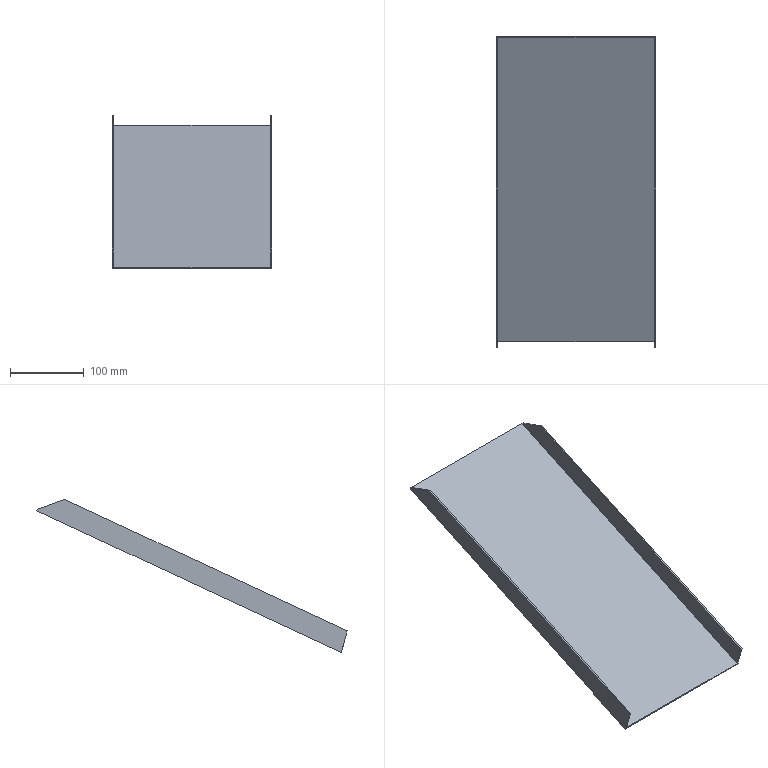Part | NX | features solid 2 | 1 solid | 12 faces | box 215.794 x 420.574 x 207.796 mm | volume 245564 mm3 | plane 12
STEP:
#1=CARTESIAN_POINT('',(-797.,-611.432,-520.479));
#2=VERTEX_POINT('',#1);
#3=CARTESIAN_POINT('',(-1008.794,-611.432,-520.479));
#4=VERTEX_POINT('',#3);
#5=CARTESIAN_POINT('',(-695.111,-611.432,-520.479));
#6=DIRECTION('',(-1.,0.,0.));
#7=VECTOR('',#6,1000.);
#8=LINE('',#5,#7);
#9=EDGE_CURVE('',#2,#4,#8,.T.);
#10=ORIENTED_EDGE('',*,*,#9,.F.);
#11=CARTESIAN_POINT('',(-797.,-199.062,-328.187));
#12=VERTEX_POINT('',#11);
#13=CARTESIAN_POINT('',(-797.,-199.062,-328.187));
#14=DIRECTION('',(0.,-0.9063,-0.4226));
#15=VECTOR('',#14,1000.);
#16=LINE('',#13,#15);
#17=EDGE_CURVE('',#12,#2,#16,.T.);
#18=ORIENTED_EDGE('',*,*,#17,.F.);
#19=CARTESIAN_POINT('',(-1008.794,-199.062,-328.187));
#20=VERTEX_POINT('',#19);
#21=CARTESIAN_POINT('',(-695.111,-199.062,-328.187));
#22=DIRECTION('',(-1.,0.,0.));
#23=VECTOR('',#22,1000.);
#24=LINE('',#21,#23);
#25=EDGE_CURVE('',#12,#20,#24,.T.);
#26=ORIENTED_EDGE('',*,*,#25,.T.);
#27=CARTESIAN_POINT('',(-1008.794,-199.062,-328.187));
#28=DIRECTION('',(0.,-0.9063,-0.4226));
#29=VECTOR('',#28,1000.);
#30=LINE('',#27,#29);
#31=EDGE_CURVE('',#20,#4,#30,.T.);
#32=ORIENTED_EDGE('',*,*,#31,.T.);
#33=EDGE_LOOP('',(#10,#18,#26,#32));
#34=FACE_BOUND('',#33,.T.);
#35=CARTESIAN_POINT('',(-695.111,-199.062,-328.187));
#36=DIRECTION('',(0.,-0.4226,0.9063));
#37=DIRECTION('',(1.,0.,0.));
#38=AXIS2_PLACEMENT_3D('',#35,#36,#37);
#39=PLANE('',#38);
#40=ADVANCED_FACE('',(#34),#39,.T.);
#41=CARTESIAN_POINT('',(-795.,-236.272,-314.644));
#42=VERTEX_POINT('',#41);
#43=CARTESIAN_POINT('',(-795.,-618.791,-493.016));
#44=VERTEX_POINT('',#43);
#45=CARTESIAN_POINT('',(-795.,-316.694,-352.146));
#46=DIRECTION('',(0.,-0.9063,-0.4226));
#47=VECTOR('',#46,1000.);
#48=LINE('',#45,#47);
#49=EDGE_CURVE('',#42,#44,#48,.T.);
#50=ORIENTED_EDGE('',*,*,#49,.T.);
#51=CARTESIAN_POINT('',(-795.,-610.906,-522.44));
#52=VERTEX_POINT('',#51);
#53=CARTESIAN_POINT('',(-795.,-682.185,-256.424));
#54=DIRECTION('',(0.,0.2588,-0.9659));
#55=VECTOR('',#54,1000.);
#56=LINE('',#53,#55);
#57=EDGE_CURVE('',#44,#52,#56,.T.);
#58=ORIENTED_EDGE('',*,*,#57,.T.);
#59=CARTESIAN_POINT('',(-795.,-198.216,-330.));
#60=VERTEX_POINT('',#59);
#61=CARTESIAN_POINT('',(-795.,-198.216,-330.));
#62=DIRECTION('',(0.,-0.9063,-0.4226));
#63=VECTOR('',#62,1000.);
#64=LINE('',#61,#63);
#65=EDGE_CURVE('',#60,#52,#64,.T.);
#66=ORIENTED_EDGE('',*,*,#65,.F.);
#67=CARTESIAN_POINT('',(-795.,-199.062,-328.187));
#68=VERTEX_POINT('',#67);
#69=CARTESIAN_POINT('',(-795.,-199.062,-328.187));
#70=DIRECTION('',(0.,0.4226,-0.9063));
#71=VECTOR('',#70,1000.);
#72=LINE('',#69,#71);
#73=EDGE_CURVE('',#68,#60,#72,.T.);
#74=ORIENTED_EDGE('',*,*,#73,.F.);
#75=CARTESIAN_POINT('',(-795.,-236.272,-314.644));
#76=DIRECTION('',(0.,0.9397,-0.342));
#77=VECTOR('',#76,1000.);
#78=LINE('',#75,#77);
#79=EDGE_CURVE('',#68,#42,#78,.F.);
#80=ORIENTED_EDGE('',*,*,#79,.T.);
#81=EDGE_LOOP('',(#50,#58,#66,#74,#80));
#82=FACE_BOUND('',#81,.T.);
#83=CARTESIAN_POINT('',(-795.,-396.967,-180.));
#84=DIRECTION('',(-1.,0.,0.));
#85=DIRECTION('',(0.,-1.,0.));
#86=AXIS2_PLACEMENT_3D('',#83,#84,#85);
#87=PLANE('',#86);
#88=ADVANCED_FACE('',(#82),#87,.F.);
#89=ORIENTED_EDGE('',*,*,#25,.F.);
#90=CARTESIAN_POINT('',(-695.111,-199.062,-328.187));
#91=DIRECTION('',(-1.,0.,0.));
#92=VECTOR('',#91,1000.);
#93=LINE('',#90,#92);
#94=EDGE_CURVE('',#68,#12,#93,.T.);
#95=ORIENTED_EDGE('',*,*,#94,.F.);
#96=ORIENTED_EDGE('',*,*,#73,.T.);
#97=CARTESIAN_POINT('',(-1010.794,-198.216,-330.));
#98=VERTEX_POINT('',#97);
#99=CARTESIAN_POINT('',(-695.111,-198.216,-330.));
#100=DIRECTION('',(-1.,0.,0.));
#101=VECTOR('',#100,1000.);
#102=LINE('',#99,#101);
#103=EDGE_CURVE('',#60,#98,#102,.T.);
#104=ORIENTED_EDGE('',*,*,#103,.T.);
#105=CARTESIAN_POINT('',(-1010.794,-199.062,-328.187));
#106=VERTEX_POINT('',#105);
#107=CARTESIAN_POINT('',(-1010.794,-199.062,-328.187));
#108=DIRECTION('',(0.,0.4226,-0.9063));
#109=VECTOR('',#108,1000.);
#110=LINE('',#107,#109);
#111=EDGE_CURVE('',#106,#98,#110,.T.);
#112=ORIENTED_EDGE('',*,*,#111,.F.);
#113=CARTESIAN_POINT('',(-1010.794,-199.062,-328.187));
#114=DIRECTION('',(-1.,0.,0.));
#115=VECTOR('',#114,1000.);
#116=LINE('',#113,#115);
#117=EDGE_CURVE('',#106,#20,#116,.F.);
#118=ORIENTED_EDGE('',*,*,#117,.T.);
#119=EDGE_LOOP('',(#89,#95,#96,#104,#112,#118));
#120=FACE_BOUND('',#119,.T.);
#121=CARTESIAN_POINT('',(-695.111,-199.062,-328.187));
#122=DIRECTION('',(0.,-0.9063,-0.4226));
#123=DIRECTION('',(0.,0.4226,-0.9063));
#124=AXIS2_PLACEMENT_3D('',#121,#122,#123);
#125=PLANE('',#124);
#126=ADVANCED_FACE('',(#120),#125,.F.);
#127=CARTESIAN_POINT('',(-1010.794,-610.906,-522.44));
#128=VERTEX_POINT('',#127);
#129=CARTESIAN_POINT('',(-1010.794,-198.216,-330.));
#130=DIRECTION('',(0.,-0.9063,-0.4226));
#131=VECTOR('',#130,1000.);
#132=LINE('',#129,#131);
#133=EDGE_CURVE('',#98,#128,#132,.T.);
#134=ORIENTED_EDGE('',*,*,#133,.T.);
#135=CARTESIAN_POINT('',(-1010.794,-618.791,-493.016));
#136=VERTEX_POINT('',#135);
#137=CARTESIAN_POINT('',(-1010.794,-631.881,-444.161));
#138=DIRECTION('',(0.,-0.2588,0.9659));
#139=VECTOR('',#138,1000.);
#140=LINE('',#137,#139);
#141=EDGE_CURVE('',#128,#136,#140,.T.);
#142=ORIENTED_EDGE('',*,*,#141,.T.);
#143=CARTESIAN_POINT('',(-1010.794,-236.272,-314.644));
#144=VERTEX_POINT('',#143);
#145=CARTESIAN_POINT('',(-1010.794,-210.895,-302.811));
#146=DIRECTION('',(0.,-0.9063,-0.4226));
#147=VECTOR('',#146,1000.);
#148=LINE('',#145,#147);
#149=EDGE_CURVE('',#144,#136,#148,.T.);
#150=ORIENTED_EDGE('',*,*,#149,.F.);
#151=CARTESIAN_POINT('',(-1010.794,-197.733,-328.671));
#152=DIRECTION('',(0.,-0.9397,0.342));
#153=VECTOR('',#152,1000.);
#154=LINE('',#151,#153);
#155=EDGE_CURVE('',#144,#106,#154,.F.);
#156=ORIENTED_EDGE('',*,*,#155,.T.);
#157=ORIENTED_EDGE('',*,*,#111,.T.);
#158=EDGE_LOOP('',(#134,#142,#150,#156,#157));
#159=FACE_BOUND('',#158,.T.);
#160=CARTESIAN_POINT('',(-1010.794,-199.062,-328.187));
#161=DIRECTION('',(1.,0.,0.));
#162=DIRECTION('',(0.,0.,-1.));
#163=AXIS2_PLACEMENT_3D('',#160,#161,#162);
#164=PLANE('',#163);
#165=ADVANCED_FACE('',(#159),#164,.F.);
#166=ORIENTED_EDGE('',*,*,#65,.T.);
#167=CARTESIAN_POINT('',(-695.111,-610.906,-522.44));
#168=DIRECTION('',(-1.,0.,0.));
#169=VECTOR('',#168,1000.);
#170=LINE('',#167,#169);
#171=EDGE_CURVE('',#52,#128,#170,.T.);
#172=ORIENTED_EDGE('',*,*,#171,.T.);
#173=ORIENTED_EDGE('',*,*,#133,.F.);
#174=ORIENTED_EDGE('',*,*,#103,.F.);
#175=EDGE_LOOP('',(#166,#172,#173,#174));
#176=FACE_BOUND('',#175,.T.);
#177=CARTESIAN_POINT('',(-695.111,-198.216,-330.));
#178=DIRECTION('',(0.,-0.4226,0.9063));
#179=DIRECTION('',(1.,0.,0.));
#180=AXIS2_PLACEMENT_3D('',#177,#178,#179);
#181=PLANE('',#180);
#182=ADVANCED_FACE('',(#176),#181,.F.);
#183=CARTESIAN_POINT('',(-1008.794,-618.791,-493.016));
#184=VERTEX_POINT('',#183);
#185=CARTESIAN_POINT('',(-1010.794,-618.791,-493.016));
#186=DIRECTION('',(1.,0.,0.));
#187=VECTOR('',#186,1000.);
#188=LINE('',#185,#187);
#189=EDGE_CURVE('',#184,#136,#188,.F.);
#190=ORIENTED_EDGE('',*,*,#189,.F.);
#191=CARTESIAN_POINT('',(-1008.794,-236.272,-314.644));
#192=VERTEX_POINT('',#191);
#193=CARTESIAN_POINT('',(-1008.794,-210.895,-302.811));
#194=DIRECTION('',(0.,-0.9063,-0.4226));
#195=VECTOR('',#194,1000.);
#196=LINE('',#193,#195);
#197=EDGE_CURVE('',#192,#184,#196,.T.);
#198=ORIENTED_EDGE('',*,*,#197,.F.);
#199=CARTESIAN_POINT('',(-1010.794,-236.272,-314.644));
#200=DIRECTION('',(1.,0.,0.));
#201=VECTOR('',#200,1000.);
#202=LINE('',#199,#201);
#203=EDGE_CURVE('',#192,#144,#202,.F.);
#204=ORIENTED_EDGE('',*,*,#203,.T.);
#205=ORIENTED_EDGE('',*,*,#149,.T.);
#206=EDGE_LOOP('',(#190,#198,#204,#205));
#207=FACE_BOUND('',#206,.T.);
#208=CARTESIAN_POINT('',(-1010.794,-210.895,-302.811));
#209=DIRECTION('',(0.,0.4226,-0.9063));
#210=DIRECTION('',(0.,-0.9063,-0.4226));
#211=AXIS2_PLACEMENT_3D('',#208,#209,#210);
#212=PLANE('',#211);
#213=ADVANCED_FACE('',(#207),#212,.F.);
#214=ORIENTED_EDGE('',*,*,#197,.T.);
#215=CARTESIAN_POINT('',(-1008.794,-631.371,-446.064));
#216=DIRECTION('',(0.,0.2588,-0.9659));
#217=VECTOR('',#216,1000.);
#218=LINE('',#215,#217);
#219=EDGE_CURVE('',#184,#4,#218,.T.);
#220=ORIENTED_EDGE('',*,*,#219,.T.);
#221=ORIENTED_EDGE('',*,*,#31,.F.);
#222=CARTESIAN_POINT('',(-1008.794,-199.062,-328.187));
#223=DIRECTION('',(0.,0.9397,-0.342));
#224=VECTOR('',#223,1000.);
#225=LINE('',#222,#224);
#226=EDGE_CURVE('',#20,#192,#225,.F.);
#227=ORIENTED_EDGE('',*,*,#226,.T.);
#228=EDGE_LOOP('',(#214,#220,#221,#227));
#229=FACE_BOUND('',#228,.T.);
#230=CARTESIAN_POINT('',(-1008.794,-198.216,-330.));
#231=DIRECTION('',(-1.,0.,0.));
#232=DIRECTION('',(0.,0.,1.));
#233=AXIS2_PLACEMENT_3D('',#230,#231,#232);
#234=PLANE('',#233);
#235=ADVANCED_FACE('',(#229),#234,.F.);
#236=ORIENTED_EDGE('',*,*,#155,.F.);
#237=ORIENTED_EDGE('',*,*,#203,.F.);
#238=ORIENTED_EDGE('',*,*,#226,.F.);
#239=ORIENTED_EDGE('',*,*,#117,.F.);
#240=EDGE_LOOP('',(#236,#237,#238,#239));
#241=FACE_BOUND('',#240,.T.);
#242=CARTESIAN_POINT('',(-1010.794,-199.062,-328.187));
#243=DIRECTION('',(0.,-0.342,-0.9397));
#244=DIRECTION('',(0.,0.9397,-0.342));
#245=AXIS2_PLACEMENT_3D('',#242,#243,#244);
#246=PLANE('',#245);
#247=ADVANCED_FACE('',(#241),#246,.F.);
#248=CARTESIAN_POINT('',(-797.,-236.272,-314.644));
#249=VERTEX_POINT('',#248);
#250=CARTESIAN_POINT('',(-797.,-618.791,-493.016));
#251=VERTEX_POINT('',#250);
#252=CARTESIAN_POINT('',(-797.,-316.694,-352.146));
#253=DIRECTION('',(0.,-0.9063,-0.4226));
#254=VECTOR('',#253,1000.);
#255=LINE('',#252,#254);
#256=EDGE_CURVE('',#249,#251,#255,.T.);
#257=ORIENTED_EDGE('',*,*,#256,.T.);
#258=CARTESIAN_POINT('',(-636.858,-618.791,-493.016));
#259=DIRECTION('',(1.,0.,0.));
#260=VECTOR('',#259,1000.);
#261=LINE('',#258,#260);
#262=EDGE_CURVE('',#251,#44,#261,.T.);
#263=ORIENTED_EDGE('',*,*,#262,.T.);
#264=ORIENTED_EDGE('',*,*,#49,.F.);
#265=CARTESIAN_POINT('',(-636.858,-236.272,-314.644));
#266=DIRECTION('',(-1.,0.,0.));
#267=VECTOR('',#266,1000.);
#268=LINE('',#265,#267);
#269=EDGE_CURVE('',#42,#249,#268,.T.);
#270=ORIENTED_EDGE('',*,*,#269,.T.);
#271=EDGE_LOOP('',(#257,#263,#264,#270));
#272=FACE_BOUND('',#271,.T.);
#273=CARTESIAN_POINT('',(-636.858,-210.895,-302.811));
#274=DIRECTION('',(0.,0.4226,-0.9063));
#275=DIRECTION('',(0.,-0.9063,-0.4226));
#276=AXIS2_PLACEMENT_3D('',#273,#274,#275);
#277=PLANE('',#276);
#278=ADVANCED_FACE('',(#272),#277,.F.);
#279=CARTESIAN_POINT('',(-797.,-682.185,-256.424));
#280=DIRECTION('',(0.,0.2588,-0.9659));
#281=VECTOR('',#280,1000.);
#282=LINE('',#279,#281);
#283=EDGE_CURVE('',#251,#2,#282,.T.);
#284=ORIENTED_EDGE('',*,*,#283,.F.);
#285=ORIENTED_EDGE('',*,*,#256,.F.);
#286=CARTESIAN_POINT('',(-797.,-421.443,-247.247));
#287=DIRECTION('',(0.,-0.9397,0.342));
#288=VECTOR('',#287,1000.);
#289=LINE('',#286,#288);
#290=EDGE_CURVE('',#249,#12,#289,.F.);
#291=ORIENTED_EDGE('',*,*,#290,.T.);
#292=ORIENTED_EDGE('',*,*,#17,.T.);
#293=EDGE_LOOP('',(#284,#285,#291,#292));
#294=FACE_BOUND('',#293,.T.);
#295=CARTESIAN_POINT('',(-797.,-396.967,-180.));
#296=DIRECTION('',(-1.,0.,0.));
#297=DIRECTION('',(0.,-1.,0.));
#298=AXIS2_PLACEMENT_3D('',#295,#296,#297);
#299=PLANE('',#298);
#300=ADVANCED_FACE('',(#294),#299,.T.);
#301=ORIENTED_EDGE('',*,*,#79,.F.);
#302=ORIENTED_EDGE('',*,*,#94,.T.);
#303=ORIENTED_EDGE('',*,*,#290,.F.);
#304=ORIENTED_EDGE('',*,*,#269,.F.);
#305=EDGE_LOOP('',(#301,#302,#303,#304));
#306=FACE_BOUND('',#305,.T.);
#307=CARTESIAN_POINT('',(-636.858,-236.272,-314.644));
#308=DIRECTION('',(0.,-0.342,-0.9397));
#309=DIRECTION('',(0.,0.9397,-0.342));
#310=AXIS2_PLACEMENT_3D('',#307,#308,#309);
#311=PLANE('',#310);
#312=ADVANCED_FACE('',(#306),#311,.F.);
#313=ORIENTED_EDGE('',*,*,#141,.F.);
#314=ORIENTED_EDGE('',*,*,#171,.F.);
#315=ORIENTED_EDGE('',*,*,#57,.F.);
#316=ORIENTED_EDGE('',*,*,#262,.F.);
#317=ORIENTED_EDGE('',*,*,#283,.T.);
#318=ORIENTED_EDGE('',*,*,#9,.T.);
#319=ORIENTED_EDGE('',*,*,#219,.F.);
#320=ORIENTED_EDGE('',*,*,#189,.T.);
#321=EDGE_LOOP('',(#313,#314,#315,#316,#317,#318,#319,#320));
#322=FACE_BOUND('',#321,.T.);
#323=CARTESIAN_POINT('',(-785.,-610.215,-525.021));
#324=DIRECTION('',(0.,0.9659,0.2588));
#325=DIRECTION('',(0.,-0.2588,0.9659));
#326=AXIS2_PLACEMENT_3D('',#323,#324,#325);
#327=PLANE('',#326);
#328=ADVANCED_FACE('',(#322),#327,.F.);
#329=CLOSED_SHELL('',(#40,#88,#126,#165,#182,#213,#235,#247,#278,#300,#312,#328));
#330=MANIFOLD_SOLID_BREP('',#329);
#331=(LENGTH_UNIT()NAMED_UNIT(*)SI_UNIT(.MILLI.,.METRE.));
#332=UNCERTAINTY_MEASURE_WITH_UNIT(LENGTH_MEASURE(0.00001),#331,'','');
#333=(NAMED_UNIT(*)PLANE_ANGLE_UNIT()SI_UNIT($,.RADIAN.));
#334=(NAMED_UNIT(*)SI_UNIT($,.STERADIAN.)SOLID_ANGLE_UNIT());
#335=(GEOMETRIC_REPRESENTATION_CONTEXT(3)GLOBAL_UNCERTAINTY_ASSIGNED_CONTEXT((#332))GLOBAL_UNIT_ASSIGNED_CONTEXT((#331,#333,#334))REPRESENTATION_CONTEXT('',''));
#336=ADVANCED_BREP_SHAPE_REPRESENTATION('',(#330),#335);